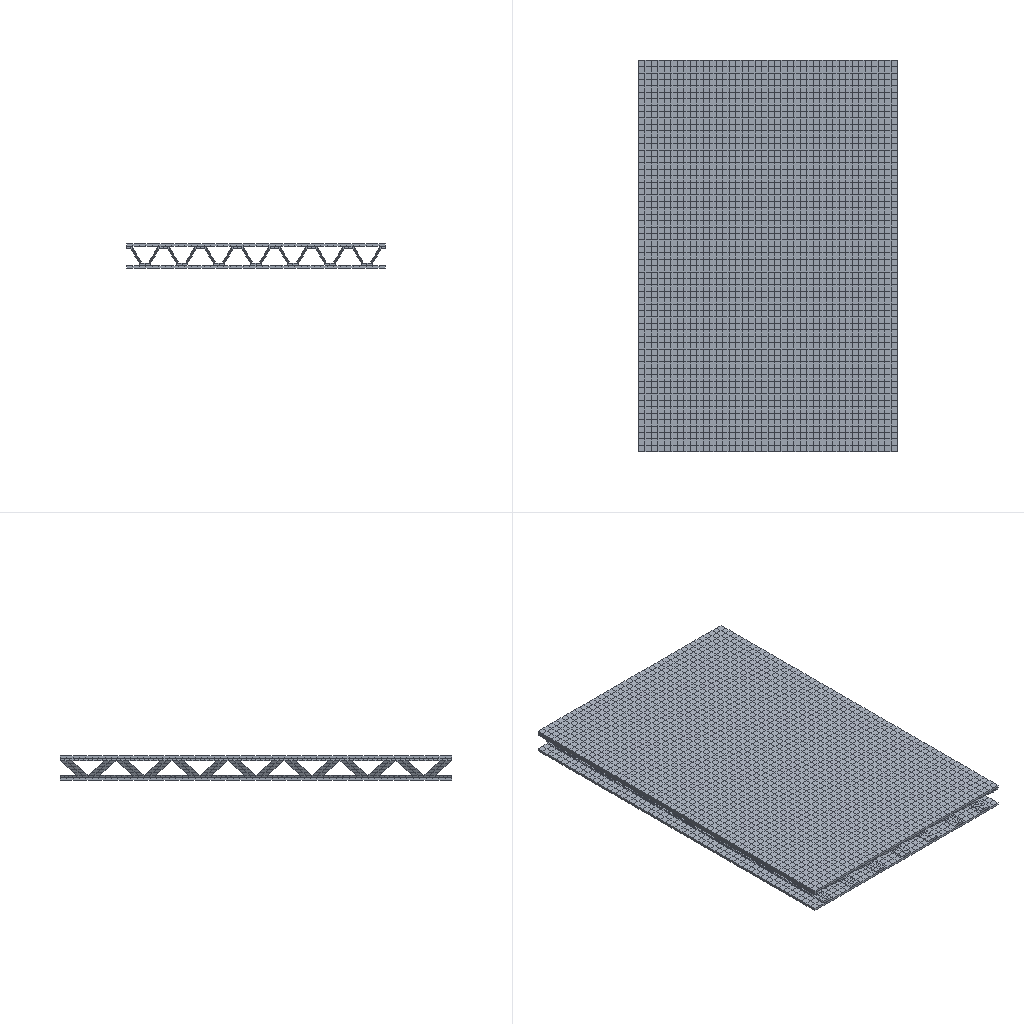Simulation study | abaqus
Set-up summary:
category,name,step,type,value,unit,region
solver,abaqus
solver,version,,,Abaqus/Standard 2020
units,not stated in the deck,,not stated
analysis,deck,,coupled temperature-displacement,coupled temperature-displacement
load_step,Step-1,Step-1,coupled temperature-displacement,nlgeom=True
contact,interactions,,,general=0 pairs=0 ties=2
load_step,requested,,,1
mesh,nodes,,,25694
mesh,elements,,,11046
element_type,C3D8RT,,solid,11046
load,load commands in deck,,count,3
bc,support commands in deck,,count,4
material,MATERIAL-1,,in results
check,setup vs results,,match,"per instance, exact: element labels, types and connectivity; labels of the nodes the elements use; coordinates of those nodes at SINGLE_PRECISION in 3 of 3 instance(s)"
Abaqus input file, long lists of numbers shortened:
*Heading
** Job name: Job-1 Model name: Job-3
** Generated by: Abaqus/CAE 2020
*Preprint, echo=NO, model=NO, history=NO, contact=NO
**
** PARTS
**
*Part, name=P1-1
*Node
      1,   125.11,   211.663,   30.427
      2,   125.11,    218.734,   30.427
** (15524 more lines like these left out)
*Element, type=C3D8RT
 1, 1606, 8863, 1597,    1, 1613, 8867, 1612,    8
 2, 8863, 1598,    2, 1597, 8867, 1611,    7, 1612
** (6164 more lines like these left out)
*Nset, nset=Set-5, generate
     1,  15526,      1
*Elset, elset=Set-5, generate
    1,  6166,     1
** Section: Section-1-_PICKEDSET3
*Solid Section, elset=Set-5, material=MATERIAL-1
,
*End Part
**
*Part, name=P1-2
*Node
      1,   132.956,   229.127,   27.427
      2,   128.914,   229.127,   27.427
** (5082 more lines like these left out)
*Element, type=C3D8RT
   1,   83,   84,  125,  124,    1,    2,   43,   42
   2,   84,   85,  126,  125,    2,    3,   44,   43
** (2438 more lines like these left out)
*Nset, nset=Set-1, generate
    1,  5084,     1
*Elset, elset=Set-1, generate
    1,  2440,     1
** Section: Section-1-_PICKEDSET3
*Solid Section, elset=Set-1, material=MATERIAL-1
,
*End Part
**
*Part, name=P1-3
*Node
      1,   132.956,   229.127,   40.927
      2,   128.914,   229.127,   40.927
** (5082 more lines like these left out)
*Element, type=C3D8RT
   1,   83,   84,  125,  124,    1,    2,   43,   42
   2,   84,   85,  126,  125,    2,    3,   44,   43
** (2438 more lines like these left out)
*Nset, nset=Set-1, generate
    1,  5084,     1
*Elset, elset=Set-1, generate
    1,  2440,     1
** Section: Section-1-_PICKEDSET3
*Solid Section, elset=Set-1, material=MATERIAL-1
,
*End Part
**
**
** ASSEMBLY
**
*Assembly, name=Assembly
**
*Instance, name=P1-1-1, part=P1-1
*End Instance
**
*Instance, name=P1-2-1, part=P1-2
*End Instance
**
*Instance, name=P1-3-1, part=P1-3
*End Instance
**
*Nset, nset=Set-38, instance=P1-1-1, generate
     1,  15526,      1
*Nset, nset=Set-38, instance=P1-2-1, generate
    1,  5084,     1
*Nset, nset=Set-38, instance=P1-3-1, generate
    1,  5084,     1
*Elset, elset=Set-38, instance=P1-1-1, generate
    1,  6166,     1
*Elset, elset=Set-38, instance=P1-2-1, generate
    1,  2440,     1
*Elset, elset=Set-38, instance=P1-3-1, generate
    1,  2440,     1
*Nset, nset=Set-39, instance=P1-2-1
    1,    2,    3,    4,    5,    6,    7,    8,    9,   10,   11,   12,   13,   14,   15,   16
   17,   18,   19,   20,   21,   22,   23,   24,   25,   26,   27,   28,   29,   30,   31,   32
** (157 more lines like these left out)
*Elset, elset=Set-39, instance=P1-2-1, generate
    1,  2440,     1
*Nset, nset=Set-40, instance=P1-3-1
   42,   43,   44,   45,   46,   47,   48,   49,   50,   51,   52,   53,   54,   55,   56,   57
   58,   59,   60,   61,   62,   63,   64,   65,   66,   67,   68,   69,   70,   71,   72,   73
** (157 more lines like these left out)
*Elset, elset=Set-40, instance=P1-3-1, generate
    1,  2440,     1
*Elset, elset=_Surf-19_S5, internal, instance=P1-2-1, generate
    1,  2440,     1
*Elset, elset=_Surf-19_S3, internal, instance=P1-3-1, generate
    1,  2440,     1
*Surface, type=ELEMENT, name=Surf-19
_Surf-19_S5, S5
_Surf-19_S3, S3
*Elset, elset=_Surf-20_S5, internal, instance=P1-3-1, generate
    1,  2440,     1
*Surface, type=ELEMENT, name=Surf-20
_Surf-20_S5, S5
*Elset, elset=_m_Surf-15_S5, internal, instance=P1-2-1, generate
    1,  2440,     1
*Surface, type=ELEMENT, name=m_Surf-15
_m_Surf-15_S5, S5
*Elset, elset=_m_Surf-17_S2, internal, instance=P1-1-1
  141,  142,  143,  144,  145,  146,  147,  148,  149,  150,  151,  152,  153,  154,  155,  156
  157,  158,  159,  160,  161,  162,  163,  164,  165,  166,  167,  168,  169,  170,  171,  172
** (144 more lines like these left out)
*Surface, type=ELEMENT, name=m_Surf-17
_m_Surf-17_S2, S2
*Elset, elset=_s_Surf-15_S2, internal, instance=P1-1-1
  468,  469,  470,  471,  472,  473,  474,  475,  476,  477,  478,  479,  480,  481,  482,  483
  484,  485,  486,  487,  488,  489,  490,  491,  492,  493,  494,  495,  496,  497,  498,  499
** (116 more lines like these left out)
*Surface, type=ELEMENT, name=s_Surf-15
_s_Surf-15_S2, S2
*Elset, elset=_s_Surf-17_S3, internal, instance=P1-3-1, generate
    1,  2440,     1
*Surface, type=ELEMENT, name=s_Surf-17
_s_Surf-17_S3, S3
** Constraint: Constraint-1
*Tie, name=Constraint-1, adjust=yes
s_Surf-15, m_Surf-15
** Constraint: Constraint-2
*Tie, name=Constraint-2, adjust=yes
s_Surf-17, m_Surf-17
*End Assembly
**
** MATERIALS
**
*Material, name=MATERIAL-1
*Conductivity
95., 298.
82., 376.
76., 496.
64., 576.
60., 698.
55., 776.
52., 896.
50., 982.
55.,1063.
48.,1163.
47.,1273.
46.,1373.
45.,1476.
*Density
 2e-09,
*Elastic
220000., 0.14
*Expansion
 2e-06,
*Specific Heat
 1.42e+09,
**
** INTERACTION PROPERTIES
**
*Film Property, name=INTPROP-1
2e-08, 298.
**
** PHYSICAL CONSTANTS
**
*Physical Constants, absolute zero=-273., stefan boltzmann=5.67e-11
**
** PREDEFINED FIELDS
**
** Name: Predefined Field-1   Type: Temperature
*Initial Conditions, type=TEMPERATURE
Set-38, 298.
** ----------------------------------------------------------------
**
** STEP: Step-1
**
*Step, name=Step-1, nlgeom=YES, inc=10000
*Coupled Temperature-displacement, creep=none, deltmx=1e+09
1., 10000., 1e-05, 1000.
**
** BOUNDARY CONDITIONS
**
** Name: BC-1 Type: 温度
*Boundary
Set-39, 11, 11, 600.
** Name: [REDACTED] Symmetric / antisymmetric / fully fixed
*Boundary
Set-40, ENCASTRE
**
** INTERACTIONS
**
** Interaction: Int-1
*Sradiate
Surf-19, AVG, 0.0, 0.8
** Interaction: Int-2
*Sfilm
Surf-20, F, 20., 0.02
**
** OUTPUT REQUESTS
**
*Restart, write, frequency=0
**
** FIELD OUTPUT: F-Output-1
**
*Output, field
*Node Output
CF, NT, RF, RM, RT, U, V
*Element Output, directions=YES
E, HFL, LE, MISES, MISESMAX, MISESONLY, NE, PE, PEEQ, PEEQMAX, PEEQT, PRESSONLY, S, SEQUT, SSAVG, TEMP
YIELDPOT
*Contact Output
CDISP, CDSTRESS, CFORCE, CNAREA, CSTATUS, CSTRESS, CSTRESSETOS, PPRESS
*Radiation Output
FTEMP,
**
** HISTORY OUTPUT: H-Output-2
**
*Output, history
*Radiation Output
FTEMP,
**
** HISTORY OUTPUT: H-Output-1
**
*Output, history, variable=PRESELECT
*End Step
Results summary:
result,step,,completed,increments=28 time=10000.0/10000.0
result,analysis,,,"coupled temperature-displacement, steady state"
result,last_loadstep,,,1
result,analysis steps,,count,1
result,primary field,,,"U, NT11"
result,reaction total,,FX,-0.000108,model units
result,reaction total,,FY,6.2e-05,model units
result,reaction total,,FZ,5e-05,model units